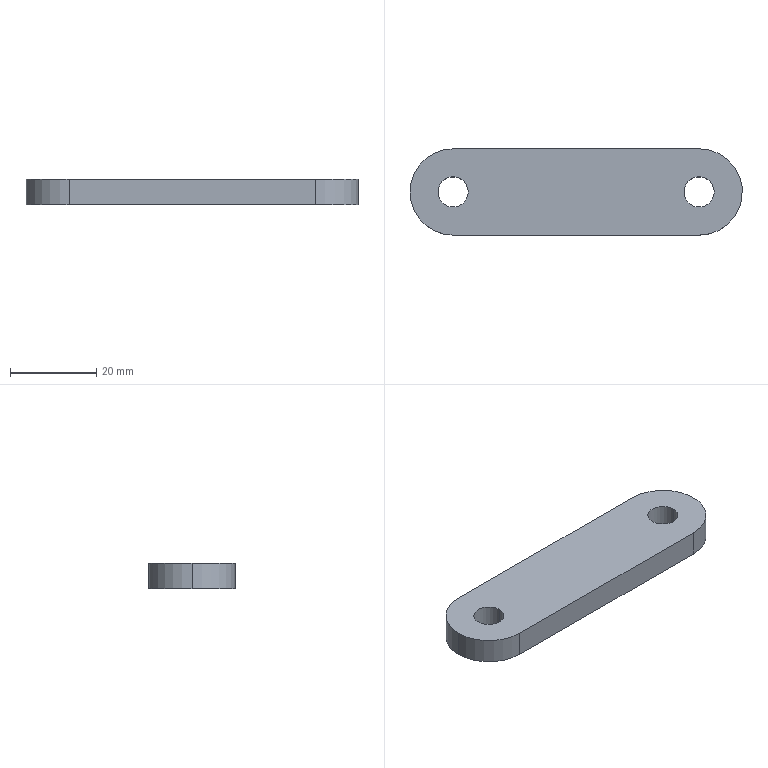Part | SolidWorks | features Extrusion 1, ICE 1 | 1 solid | 11 faces | box 77.02 x 20 x 6 mm | volume 8266 mm3 | cylinder 7 | plane 4 | commonest cylinder face diameters 7 x4 20 x3
STEP:
#1=CARTESIAN_POINT('',(53.52,0.,0.));
#2=VERTEX_POINT('',#1);
#3=CARTESIAN_POINT('',(60.52,0.,0.));
#4=VERTEX_POINT('',#3);
#5=CARTESIAN_POINT('',(57.02,0.,0.));
#6=DIRECTION('',(0.,0.,1.));
#7=DIRECTION('',(1.,0.,0.));
#8=AXIS2_PLACEMENT_3D('',#5,#6,#7);
#9=CIRCLE('',#8,3.5);
#10=EDGE_CURVE('',#2,#4,#9,.T.);
#11=ORIENTED_EDGE('',*,*,#10,.F.);
#12=CARTESIAN_POINT('',(53.52,0.,6.));
#13=VERTEX_POINT('',#12);
#14=CARTESIAN_POINT('',(53.52,0.,-89.));
#15=DIRECTION('',(0.,0.,1.));
#16=VECTOR('',#15,1000.);
#17=LINE('',#14,#16);
#18=EDGE_CURVE('',#2,#13,#17,.T.);
#19=ORIENTED_EDGE('',*,*,#18,.T.);
#20=CARTESIAN_POINT('',(60.52,0.,6.));
#21=VERTEX_POINT('',#20);
#22=CARTESIAN_POINT('',(57.02,0.,6.));
#23=DIRECTION('',(0.,0.,1.));
#24=DIRECTION('',(1.,0.,0.));
#25=AXIS2_PLACEMENT_3D('',#22,#23,#24);
#26=CIRCLE('',#25,3.5);
#27=EDGE_CURVE('',#13,#21,#26,.T.);
#28=ORIENTED_EDGE('',*,*,#27,.T.);
#29=CARTESIAN_POINT('',(60.52,0.,-89.));
#30=DIRECTION('',(0.,0.,1.));
#31=VECTOR('',#30,1000.);
#32=LINE('',#29,#31);
#33=EDGE_CURVE('',#4,#21,#32,.T.);
#34=ORIENTED_EDGE('',*,*,#33,.F.);
#35=EDGE_LOOP('',(#11,#19,#28,#34));
#36=FACE_OUTER_BOUND('',#35,.T.);
#37=CARTESIAN_POINT('',(57.02,0.,-89.));
#38=DIRECTION('',(0.,0.,1.));
#39=DIRECTION('',(1.,0.,0.));
#40=AXIS2_PLACEMENT_3D('',#37,#38,#39);
#41=CYLINDRICAL_SURFACE('',#40,3.5);
#42=ADVANCED_FACE('',(#36),#41,.F.);
#43=CARTESIAN_POINT('',(-3.5,0.,0.));
#44=VERTEX_POINT('',#43);
#45=CARTESIAN_POINT('',(3.5,0.,0.));
#46=VERTEX_POINT('',#45);
#47=CARTESIAN_POINT('',(0.,0.,0.));
#48=DIRECTION('',(0.,0.,1.));
#49=DIRECTION('',(1.,0.,0.));
#50=AXIS2_PLACEMENT_3D('',#47,#48,#49);
#51=CIRCLE('',#50,3.5);
#52=EDGE_CURVE('',#44,#46,#51,.T.);
#53=ORIENTED_EDGE('',*,*,#52,.F.);
#54=CARTESIAN_POINT('',(-3.5,0.,6.));
#55=VERTEX_POINT('',#54);
#56=CARTESIAN_POINT('',(-3.5,0.,-89.));
#57=DIRECTION('',(0.,0.,1.));
#58=VECTOR('',#57,1000.);
#59=LINE('',#56,#58);
#60=EDGE_CURVE('',#44,#55,#59,.T.);
#61=ORIENTED_EDGE('',*,*,#60,.T.);
#62=CARTESIAN_POINT('',(3.5,0.,6.));
#63=VERTEX_POINT('',#62);
#64=CARTESIAN_POINT('',(0.,0.,6.));
#65=DIRECTION('',(0.,0.,1.));
#66=DIRECTION('',(1.,0.,0.));
#67=AXIS2_PLACEMENT_3D('',#64,#65,#66);
#68=CIRCLE('',#67,3.5);
#69=EDGE_CURVE('',#55,#63,#68,.T.);
#70=ORIENTED_EDGE('',*,*,#69,.T.);
#71=CARTESIAN_POINT('',(3.5,0.,-89.));
#72=DIRECTION('',(0.,0.,1.));
#73=VECTOR('',#72,1000.);
#74=LINE('',#71,#73);
#75=EDGE_CURVE('',#46,#63,#74,.T.);
#76=ORIENTED_EDGE('',*,*,#75,.F.);
#77=EDGE_LOOP('',(#53,#61,#70,#76));
#78=FACE_OUTER_BOUND('',#77,.T.);
#79=CARTESIAN_POINT('',(0.,0.,-89.));
#80=DIRECTION('',(0.,0.,1.));
#81=DIRECTION('',(1.,0.,0.));
#82=AXIS2_PLACEMENT_3D('',#79,#80,#81);
#83=CYLINDRICAL_SURFACE('',#82,3.5);
#84=ADVANCED_FACE('',(#78),#83,.F.);
#85=CARTESIAN_POINT('',(-10.,0.,6.));
#86=VERTEX_POINT('',#85);
#87=CARTESIAN_POINT('',(0.,-10.,6.));
#88=VERTEX_POINT('',#87);
#89=CARTESIAN_POINT('',(0.,0.,6.));
#90=DIRECTION('',(0.,0.,1.));
#91=DIRECTION('',(1.,0.,0.));
#92=AXIS2_PLACEMENT_3D('',#89,#90,#91);
#93=CIRCLE('',#92,10.);
#94=EDGE_CURVE('',#86,#88,#93,.T.);
#95=ORIENTED_EDGE('',*,*,#94,.F.);
#96=CARTESIAN_POINT('',(-10.,0.,0.));
#97=VERTEX_POINT('',#96);
#98=CARTESIAN_POINT('',(-10.,0.,6.));
#99=DIRECTION('',(0.,0.,-1.));
#100=VECTOR('',#99,1000.);
#101=LINE('',#98,#100);
#102=EDGE_CURVE('',#86,#97,#101,.T.);
#103=ORIENTED_EDGE('',*,*,#102,.T.);
#104=CARTESIAN_POINT('',(0.,-10.,0.));
#105=VERTEX_POINT('',#104);
#106=CARTESIAN_POINT('',(0.,0.,0.));
#107=DIRECTION('',(0.,0.,1.));
#108=DIRECTION('',(1.,0.,0.));
#109=AXIS2_PLACEMENT_3D('',#106,#107,#108);
#110=CIRCLE('',#109,10.);
#111=EDGE_CURVE('',#97,#105,#110,.T.);
#112=ORIENTED_EDGE('',*,*,#111,.T.);
#113=CARTESIAN_POINT('',(0.,-10.,6.));
#114=DIRECTION('',(0.,0.,-1.));
#115=VECTOR('',#114,1000.);
#116=LINE('',#113,#115);
#117=EDGE_CURVE('',#88,#105,#116,.T.);
#118=ORIENTED_EDGE('',*,*,#117,.F.);
#119=EDGE_LOOP('',(#95,#103,#112,#118));
#120=FACE_OUTER_BOUND('',#119,.T.);
#121=CARTESIAN_POINT('',(0.,0.,6.));
#122=DIRECTION('',(0.,0.,-1.));
#123=DIRECTION('',(-1.,0.,0.));
#124=AXIS2_PLACEMENT_3D('',#121,#122,#123);
#125=CYLINDRICAL_SURFACE('',#124,10.);
#126=ADVANCED_FACE('',(#120),#125,.T.);
#127=ORIENTED_EDGE('',*,*,#102,.F.);
#128=CARTESIAN_POINT('',(0.,10.,6.));
#129=VERTEX_POINT('',#128);
#130=CARTESIAN_POINT('',(0.,0.,6.));
#131=DIRECTION('',(0.,0.,1.));
#132=DIRECTION('',(1.,0.,0.));
#133=AXIS2_PLACEMENT_3D('',#130,#131,#132);
#134=CIRCLE('',#133,10.);
#135=EDGE_CURVE('',#129,#86,#134,.T.);
#136=ORIENTED_EDGE('',*,*,#135,.F.);
#137=CARTESIAN_POINT('',(0.,10.,0.));
#138=VERTEX_POINT('',#137);
#139=CARTESIAN_POINT('',(0.,10.,6.));
#140=DIRECTION('',(0.,0.,-1.));
#141=VECTOR('',#140,1000.);
#142=LINE('',#139,#141);
#143=EDGE_CURVE('',#129,#138,#142,.T.);
#144=ORIENTED_EDGE('',*,*,#143,.T.);
#145=CARTESIAN_POINT('',(0.,0.,0.));
#146=DIRECTION('',(0.,0.,1.));
#147=DIRECTION('',(1.,0.,0.));
#148=AXIS2_PLACEMENT_3D('',#145,#146,#147);
#149=CIRCLE('',#148,10.);
#150=EDGE_CURVE('',#138,#97,#149,.T.);
#151=ORIENTED_EDGE('',*,*,#150,.T.);
#152=EDGE_LOOP('',(#127,#136,#144,#151));
#153=FACE_OUTER_BOUND('',#152,.T.);
#154=CARTESIAN_POINT('',(0.,0.,6.));
#155=DIRECTION('',(0.,0.,-1.));
#156=DIRECTION('',(-1.,0.,0.));
#157=AXIS2_PLACEMENT_3D('',#154,#155,#156);
#158=CYLINDRICAL_SURFACE('',#157,10.);
#159=ADVANCED_FACE('',(#153),#158,.T.);
#160=CARTESIAN_POINT('',(57.02,-10.,0.));
#161=VERTEX_POINT('',#160);
#162=CARTESIAN_POINT('',(0.,-10.,0.));
#163=DIRECTION('',(1.,0.,0.));
#164=VECTOR('',#163,1000.);
#165=LINE('',#162,#164);
#166=EDGE_CURVE('',#105,#161,#165,.T.);
#167=ORIENTED_EDGE('',*,*,#166,.T.);
#168=CARTESIAN_POINT('',(57.02,-10.,6.));
#169=VERTEX_POINT('',#168);
#170=CARTESIAN_POINT('',(57.02,-10.,6.));
#171=DIRECTION('',(0.,0.,-1.));
#172=VECTOR('',#171,1000.);
#173=LINE('',#170,#172);
#174=EDGE_CURVE('',#169,#161,#173,.T.);
#175=ORIENTED_EDGE('',*,*,#174,.F.);
#176=CARTESIAN_POINT('',(0.,-10.,6.));
#177=DIRECTION('',(1.,0.,0.));
#178=VECTOR('',#177,1000.);
#179=LINE('',#176,#178);
#180=EDGE_CURVE('',#88,#169,#179,.T.);
#181=ORIENTED_EDGE('',*,*,#180,.F.);
#182=ORIENTED_EDGE('',*,*,#117,.T.);
#183=EDGE_LOOP('',(#167,#175,#181,#182));
#184=FACE_OUTER_BOUND('',#183,.T.);
#185=CARTESIAN_POINT('',(0.,-10.,6.));
#186=DIRECTION('',(0.,1.,0.));
#187=DIRECTION('',(0.,0.,1.));
#188=AXIS2_PLACEMENT_3D('',#185,#186,#187);
#189=PLANE('',#188);
#190=ADVANCED_FACE('',(#184),#189,.F.);
#191=CARTESIAN_POINT('',(57.02,10.,0.));
#192=VERTEX_POINT('',#191);
#193=CARTESIAN_POINT('',(57.02,0.,0.));
#194=DIRECTION('',(0.,0.,1.));
#195=DIRECTION('',(1.,0.,0.));
#196=AXIS2_PLACEMENT_3D('',#193,#194,#195);
#197=CIRCLE('',#196,10.);
#198=EDGE_CURVE('',#161,#192,#197,.T.);
#199=ORIENTED_EDGE('',*,*,#198,.T.);
#200=CARTESIAN_POINT('',(57.02,10.,6.));
#201=VERTEX_POINT('',#200);
#202=CARTESIAN_POINT('',(57.02,10.,6.));
#203=DIRECTION('',(0.,0.,-1.));
#204=VECTOR('',#203,1000.);
#205=LINE('',#202,#204);
#206=EDGE_CURVE('',#201,#192,#205,.T.);
#207=ORIENTED_EDGE('',*,*,#206,.F.);
#208=CARTESIAN_POINT('',(57.02,0.,6.));
#209=DIRECTION('',(0.,0.,1.));
#210=DIRECTION('',(1.,0.,0.));
#211=AXIS2_PLACEMENT_3D('',#208,#209,#210);
#212=CIRCLE('',#211,10.);
#213=EDGE_CURVE('',#169,#201,#212,.T.);
#214=ORIENTED_EDGE('',*,*,#213,.F.);
#215=ORIENTED_EDGE('',*,*,#174,.T.);
#216=EDGE_LOOP('',(#199,#207,#214,#215));
#217=FACE_OUTER_BOUND('',#216,.T.);
#218=CARTESIAN_POINT('',(57.02,0.,6.));
#219=DIRECTION('',(0.,0.,-1.));
#220=DIRECTION('',(-1.,0.,0.));
#221=AXIS2_PLACEMENT_3D('',#218,#219,#220);
#222=CYLINDRICAL_SURFACE('',#221,10.);
#223=ADVANCED_FACE('',(#217),#222,.T.);
#224=CARTESIAN_POINT('',(0.,10.,0.));
#225=DIRECTION('',(-1.,0.,0.));
#226=VECTOR('',#225,1000.);
#227=LINE('',#224,#226);
#228=EDGE_CURVE('',#192,#138,#227,.T.);
#229=ORIENTED_EDGE('',*,*,#228,.T.);
#230=ORIENTED_EDGE('',*,*,#143,.F.);
#231=CARTESIAN_POINT('',(0.,10.,6.));
#232=DIRECTION('',(-1.,0.,0.));
#233=VECTOR('',#232,1000.);
#234=LINE('',#231,#233);
#235=EDGE_CURVE('',#201,#129,#234,.T.);
#236=ORIENTED_EDGE('',*,*,#235,.F.);
#237=ORIENTED_EDGE('',*,*,#206,.T.);
#238=EDGE_LOOP('',(#229,#230,#236,#237));
#239=FACE_OUTER_BOUND('',#238,.T.);
#240=CARTESIAN_POINT('',(0.,10.,6.));
#241=DIRECTION('',(0.,-1.,0.));
#242=DIRECTION('',(0.,0.,-1.));
#243=AXIS2_PLACEMENT_3D('',#240,#241,#242);
#244=PLANE('',#243);
#245=ADVANCED_FACE('',(#239),#244,.F.);
#246=CARTESIAN_POINT('',(57.02,0.,6.));
#247=DIRECTION('',(0.,0.,1.));
#248=DIRECTION('',(1.,0.,0.));
#249=AXIS2_PLACEMENT_3D('',#246,#247,#248);
#250=CIRCLE('',#249,3.5);
#251=EDGE_CURVE('',#21,#13,#250,.T.);
#252=ORIENTED_EDGE('',*,*,#251,.F.);
#253=ORIENTED_EDGE('',*,*,#27,.F.);
#254=EDGE_LOOP('',(#252,#253));
#255=FACE_BOUND('',#254,.T.);
#256=CARTESIAN_POINT('',(0.,0.,6.));
#257=DIRECTION('',(0.,0.,1.));
#258=DIRECTION('',(1.,0.,0.));
#259=AXIS2_PLACEMENT_3D('',#256,#257,#258);
#260=CIRCLE('',#259,3.5);
#261=EDGE_CURVE('',#63,#55,#260,.T.);
#262=ORIENTED_EDGE('',*,*,#261,.F.);
#263=ORIENTED_EDGE('',*,*,#69,.F.);
#264=EDGE_LOOP('',(#262,#263));
#265=FACE_BOUND('',#264,.T.);
#266=ORIENTED_EDGE('',*,*,#135,.T.);
#267=ORIENTED_EDGE('',*,*,#94,.T.);
#268=ORIENTED_EDGE('',*,*,#180,.T.);
#269=ORIENTED_EDGE('',*,*,#213,.T.);
#270=ORIENTED_EDGE('',*,*,#235,.T.);
#271=EDGE_LOOP('',(#266,#267,#268,#269,#270));
#272=FACE_OUTER_BOUND('',#271,.T.);
#273=CARTESIAN_POINT('',(0.,0.,6.));
#274=DIRECTION('',(0.,0.,1.));
#275=DIRECTION('',(1.,0.,0.));
#276=AXIS2_PLACEMENT_3D('',#273,#274,#275);
#277=PLANE('',#276);
#278=ADVANCED_FACE('',(#255,#265,#272),#277,.T.);
#279=CARTESIAN_POINT('',(57.02,0.,0.));
#280=DIRECTION('',(0.,0.,1.));
#281=DIRECTION('',(1.,0.,0.));
#282=AXIS2_PLACEMENT_3D('',#279,#280,#281);
#283=CIRCLE('',#282,3.5);
#284=EDGE_CURVE('',#4,#2,#283,.T.);
#285=ORIENTED_EDGE('',*,*,#284,.T.);
#286=ORIENTED_EDGE('',*,*,#10,.T.);
#287=EDGE_LOOP('',(#285,#286));
#288=FACE_BOUND('',#287,.T.);
#289=CARTESIAN_POINT('',(0.,0.,0.));
#290=DIRECTION('',(0.,0.,1.));
#291=DIRECTION('',(1.,0.,0.));
#292=AXIS2_PLACEMENT_3D('',#289,#290,#291);
#293=CIRCLE('',#292,3.5);
#294=EDGE_CURVE('',#46,#44,#293,.T.);
#295=ORIENTED_EDGE('',*,*,#294,.T.);
#296=ORIENTED_EDGE('',*,*,#52,.T.);
#297=EDGE_LOOP('',(#295,#296));
#298=FACE_BOUND('',#297,.T.);
#299=ORIENTED_EDGE('',*,*,#150,.F.);
#300=ORIENTED_EDGE('',*,*,#228,.F.);
#301=ORIENTED_EDGE('',*,*,#198,.F.);
#302=ORIENTED_EDGE('',*,*,#166,.F.);
#303=ORIENTED_EDGE('',*,*,#111,.F.);
#304=EDGE_LOOP('',(#299,#300,#301,#302,#303));
#305=FACE_OUTER_BOUND('',#304,.T.);
#306=CARTESIAN_POINT('',(0.,0.,0.));
#307=DIRECTION('',(0.,0.,1.));
#308=DIRECTION('',(1.,0.,0.));
#309=AXIS2_PLACEMENT_3D('',#306,#307,#308);
#310=PLANE('',#309);
#311=ADVANCED_FACE('',(#288,#298,#305),#310,.F.);
#312=ORIENTED_EDGE('',*,*,#60,.F.);
#313=ORIENTED_EDGE('',*,*,#294,.F.);
#314=ORIENTED_EDGE('',*,*,#75,.T.);
#315=ORIENTED_EDGE('',*,*,#261,.T.);
#316=EDGE_LOOP('',(#312,#313,#314,#315));
#317=FACE_OUTER_BOUND('',#316,.T.);
#318=CARTESIAN_POINT('',(0.,0.,-89.));
#319=DIRECTION('',(0.,0.,1.));
#320=DIRECTION('',(1.,0.,0.));
#321=AXIS2_PLACEMENT_3D('',#318,#319,#320);
#322=CYLINDRICAL_SURFACE('',#321,3.5);
#323=ADVANCED_FACE('',(#317),#322,.F.);
#324=ORIENTED_EDGE('',*,*,#18,.F.);
#325=ORIENTED_EDGE('',*,*,#284,.F.);
#326=ORIENTED_EDGE('',*,*,#33,.T.);
#327=ORIENTED_EDGE('',*,*,#251,.T.);
#328=EDGE_LOOP('',(#324,#325,#326,#327));
#329=FACE_OUTER_BOUND('',#328,.T.);
#330=CARTESIAN_POINT('',(57.02,0.,-89.));
#331=DIRECTION('',(0.,0.,1.));
#332=DIRECTION('',(1.,0.,0.));
#333=AXIS2_PLACEMENT_3D('',#330,#331,#332);
#334=CYLINDRICAL_SURFACE('',#333,3.5);
#335=ADVANCED_FACE('',(#329),#334,.F.);
#336=CLOSED_SHELL('',(#42,#84,#126,#159,#190,#223,#245,#278,#311,#323,#335));
#337=MANIFOLD_SOLID_BREP('',#336);
#338=CARTESIAN_POINT('',(0.,0.,0.));
#339=DIRECTION('',(0.,0.,1.));
#340=DIRECTION('',(1.,0.,0.));
#341=AXIS2_PLACEMENT_3D('',#338,#339,#340);
#342=(LENGTH_UNIT()NAMED_UNIT(*)SI_UNIT(.MILLI.,.METRE.));
#343=UNCERTAINTY_MEASURE_WITH_UNIT(LENGTH_MEASURE(0.00001),#342,'','');
#344=(NAMED_UNIT(*)PLANE_ANGLE_UNIT()SI_UNIT($,.RADIAN.));
#345=(NAMED_UNIT(*)SI_UNIT($,.STERADIAN.)SOLID_ANGLE_UNIT());
#346=(GEOMETRIC_REPRESENTATION_CONTEXT(3)GLOBAL_UNCERTAINTY_ASSIGNED_CONTEXT((#343))GLOBAL_UNIT_ASSIGNED_CONTEXT((#342,#344,#345))REPRESENTATION_CONTEXT('',''));
#347=ADVANCED_BREP_SHAPE_REPRESENTATION('',(#337,#341),#346);